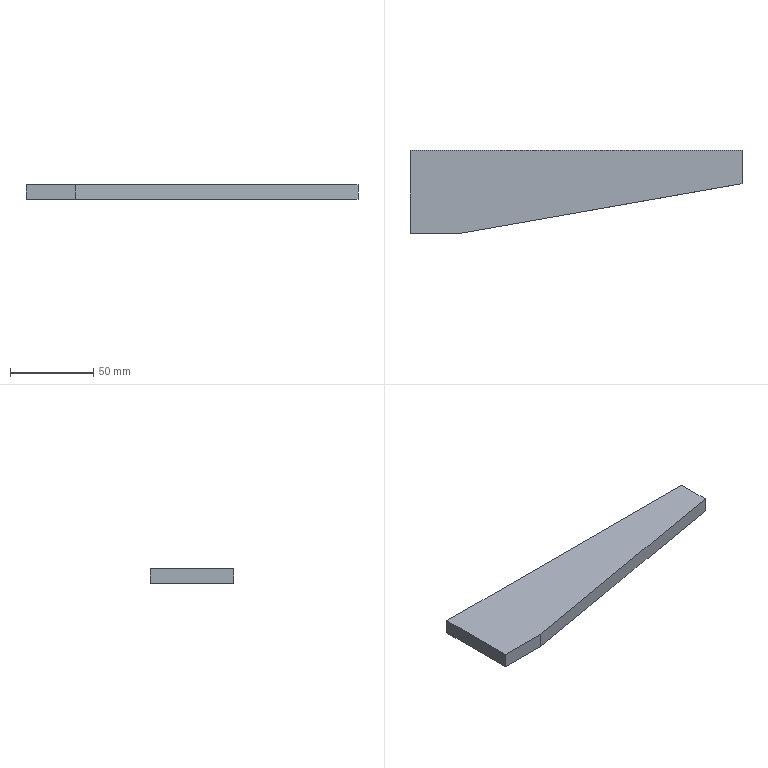Part | STEP file | [05]-1 | 1 solid | 7 faces | box 200 x 50 x 9 mm | volume 67050 mm3 | plane 7
STEP:
#1=CARTESIAN_POINT('',(0.,0.,0.));
#2=DIRECTION('',(0.,0.,1.));
#3=DIRECTION('',(1.,0.,0.));
#4=AXIS2_PLACEMENT_3D('',#1,#2,#3);
#5=CARTESIAN_POINT('',(200.,-20.,0.));
#6=VERTEX_POINT('',#5);
#7=CARTESIAN_POINT('',(200.,0.,0.));
#8=VERTEX_POINT('',#7);
#9=CARTESIAN_POINT('',(200.,-25.,0.));
#10=DIRECTION('',(0.,1.,0.));
#11=VECTOR('',#10,1.);
#12=LINE('',#9,#11);
#13=CARTESIAN_POINT('',(100.,-25.,0.));
#14=DIRECTION('',(0.,0.,-1.));
#15=DIRECTION('',(-1.,0.,0.));
#16=AXIS2_PLACEMENT_3D('',#13,#14,#15);
#17=PLANE('',#16);
#18=CARTESIAN_POINT('',(-100.,0.));
#19=DIRECTION('',(0.,1.));
#20=VECTOR('',#19,1.);
#21=LINE('',#18,#20);
#22=(GEOMETRIC_REPRESENTATION_CONTEXT(2)PARAMETRIC_REPRESENTATION_CONTEXT()REPRESENTATION_CONTEXT('',''));
#23=DEFINITIONAL_REPRESENTATION('',(#21),#22);
#24=PCURVE('',#17,#23);
#25=CARTESIAN_POINT('',(200.,-25.,9.));
#26=DIRECTION('',(1.,0.,0.));
#27=DIRECTION('',(0.,0.,-1.));
#28=AXIS2_PLACEMENT_3D('',#25,#26,#27);
#29=PLANE('',#28);
#30=CARTESIAN_POINT('',(9.,0.));
#31=DIRECTION('',(0.,1.));
#32=VECTOR('',#31,1.);
#33=LINE('',#30,#32);
#34=(GEOMETRIC_REPRESENTATION_CONTEXT(2)PARAMETRIC_REPRESENTATION_CONTEXT()REPRESENTATION_CONTEXT('',''));
#35=DEFINITIONAL_REPRESENTATION('',(#33),#34);
#36=PCURVE('',#29,#35);
#37=SURFACE_CURVE('',#12,(#24,#36),.PCURVE_S1.);
#38=EDGE_CURVE('',#6,#8,#37,.T.);
#39=ORIENTED_EDGE('',*,*,#38,.F.);
#40=CARTESIAN_POINT('',(30.,-50.,0.));
#41=VERTEX_POINT('',#40);
#42=CARTESIAN_POINT('',(102.164,-37.265,0.));
#43=DIRECTION('',(-0.9848,-0.1738,0.));
#44=VECTOR('',#43,1.);
#45=LINE('',#42,#44);
#46=CARTESIAN_POINT('',(-2.164,-12.265));
#47=DIRECTION('',(0.9848,-0.1738));
#48=VECTOR('',#47,1.);
#49=LINE('',#46,#48);
#50=(GEOMETRIC_REPRESENTATION_CONTEXT(2)PARAMETRIC_REPRESENTATION_CONTEXT()REPRESENTATION_CONTEXT('',''));
#51=DEFINITIONAL_REPRESENTATION('',(#49),#50);
#52=PCURVE('',#17,#51);
#53=CARTESIAN_POINT('',(200.,-20.,9.));
#54=DIRECTION('',(-0.1738,0.9848,0.));
#55=DIRECTION('',(0.,0.,-1.));
#56=AXIS2_PLACEMENT_3D('',#53,#54,#55);
#57=PLANE('',#56);
#58=CARTESIAN_POINT('',(9.,99.347));
#59=DIRECTION('',(0.,1.));
#60=VECTOR('',#59,1.);
#61=LINE('',#58,#60);
#62=(GEOMETRIC_REPRESENTATION_CONTEXT(2)PARAMETRIC_REPRESENTATION_CONTEXT()REPRESENTATION_CONTEXT('',''));
#63=DEFINITIONAL_REPRESENTATION('',(#61),#62);
#64=PCURVE('',#57,#63);
#65=SURFACE_CURVE('',#45,(#52,#64),.PCURVE_S1.);
#66=EDGE_CURVE('',#6,#41,#65,.T.);
#67=ORIENTED_EDGE('',*,*,#66,.T.);
#68=CARTESIAN_POINT('',(0.,-50.,0.));
#69=VERTEX_POINT('',#68);
#70=CARTESIAN_POINT('',(100.,-50.,0.));
#71=DIRECTION('',(1.,0.,0.));
#72=VECTOR('',#71,1.);
#73=LINE('',#70,#72);
#74=CARTESIAN_POINT('',(0.,-25.));
#75=DIRECTION('',(-1.,0.));
#76=VECTOR('',#75,1.);
#77=LINE('',#74,#76);
#78=(GEOMETRIC_REPRESENTATION_CONTEXT(2)PARAMETRIC_REPRESENTATION_CONTEXT()REPRESENTATION_CONTEXT('',''));
#79=DEFINITIONAL_REPRESENTATION('',(#77),#78);
#80=PCURVE('',#17,#79);
#81=CARTESIAN_POINT('',(100.,-50.,9.));
#82=DIRECTION('',(0.,-1.,0.));
#83=DIRECTION('',(0.,0.,1.));
#84=AXIS2_PLACEMENT_3D('',#81,#82,#83);
#85=PLANE('',#84);
#86=CARTESIAN_POINT('',(-9.,0.));
#87=DIRECTION('',(0.,-1.));
#88=VECTOR('',#87,1.);
#89=LINE('',#86,#88);
#90=(GEOMETRIC_REPRESENTATION_CONTEXT(2)PARAMETRIC_REPRESENTATION_CONTEXT()REPRESENTATION_CONTEXT('',''));
#91=DEFINITIONAL_REPRESENTATION('',(#89),#90);
#92=PCURVE('',#85,#91);
#93=SURFACE_CURVE('',#73,(#80,#92),.PCURVE_S1.);
#94=EDGE_CURVE('',#69,#41,#93,.T.);
#95=ORIENTED_EDGE('',*,*,#94,.F.);
#96=CARTESIAN_POINT('',(0.,0.,0.));
#97=VERTEX_POINT('',#96);
#98=CARTESIAN_POINT('',(0.,-25.,0.));
#99=DIRECTION('',(0.,-1.,0.));
#100=VECTOR('',#99,1.);
#101=LINE('',#98,#100);
#102=CARTESIAN_POINT('',(100.,0.));
#103=DIRECTION('',(0.,-1.));
#104=VECTOR('',#103,1.);
#105=LINE('',#102,#104);
#106=(GEOMETRIC_REPRESENTATION_CONTEXT(2)PARAMETRIC_REPRESENTATION_CONTEXT()REPRESENTATION_CONTEXT('',''));
#107=DEFINITIONAL_REPRESENTATION('',(#105),#106);
#108=PCURVE('',#17,#107);
#109=CARTESIAN_POINT('',(0.,-25.,9.));
#110=DIRECTION('',(-1.,0.,0.));
#111=DIRECTION('',(0.,0.,1.));
#112=AXIS2_PLACEMENT_3D('',#109,#110,#111);
#113=PLANE('',#112);
#114=CARTESIAN_POINT('',(-9.,0.));
#115=DIRECTION('',(0.,-1.));
#116=VECTOR('',#115,1.);
#117=LINE('',#114,#116);
#118=(GEOMETRIC_REPRESENTATION_CONTEXT(2)PARAMETRIC_REPRESENTATION_CONTEXT()REPRESENTATION_CONTEXT('',''));
#119=DEFINITIONAL_REPRESENTATION('',(#117),#118);
#120=PCURVE('',#113,#119);
#121=SURFACE_CURVE('',#101,(#108,#120),.PCURVE_S1.);
#122=EDGE_CURVE('',#97,#69,#121,.T.);
#123=ORIENTED_EDGE('',*,*,#122,.F.);
#124=CARTESIAN_POINT('',(100.,0.,0.));
#125=DIRECTION('',(-1.,0.,0.));
#126=VECTOR('',#125,1.);
#127=LINE('',#124,#126);
#128=CARTESIAN_POINT('',(0.,25.));
#129=DIRECTION('',(1.,0.));
#130=VECTOR('',#129,1.);
#131=LINE('',#128,#130);
#132=(GEOMETRIC_REPRESENTATION_CONTEXT(2)PARAMETRIC_REPRESENTATION_CONTEXT()REPRESENTATION_CONTEXT('',''));
#133=DEFINITIONAL_REPRESENTATION('',(#131),#132);
#134=PCURVE('',#17,#133);
#135=CARTESIAN_POINT('',(100.,0.,9.));
#136=DIRECTION('',(0.,1.,0.));
#137=DIRECTION('',(0.,0.,-1.));
#138=AXIS2_PLACEMENT_3D('',#135,#136,#137);
#139=PLANE('',#138);
#140=CARTESIAN_POINT('',(9.,0.));
#141=DIRECTION('',(0.,1.));
#142=VECTOR('',#141,1.);
#143=LINE('',#140,#142);
#144=(GEOMETRIC_REPRESENTATION_CONTEXT(2)PARAMETRIC_REPRESENTATION_CONTEXT()REPRESENTATION_CONTEXT('',''));
#145=DEFINITIONAL_REPRESENTATION('',(#143),#144);
#146=PCURVE('',#139,#145);
#147=SURFACE_CURVE('',#127,(#134,#146),.PCURVE_S1.);
#148=EDGE_CURVE('',#8,#97,#147,.T.);
#149=ORIENTED_EDGE('',*,*,#148,.F.);
#150=EDGE_LOOP('',(#39,#67,#95,#123,#149));
#151=FACE_BOUND('',#150,.T.);
#152=ADVANCED_FACE('',(#151),#17,.T.);
#153=ORIENTED_EDGE('',*,*,#94,.T.);
#154=CARTESIAN_POINT('',(30.,-50.,9.));
#155=VERTEX_POINT('',#154);
#156=CARTESIAN_POINT('',(30.,-50.,9.));
#157=DIRECTION('',(0.,0.,1.));
#158=VECTOR('',#157,1.);
#159=LINE('',#156,#158);
#160=CARTESIAN_POINT('',(0.,70.));
#161=DIRECTION('',(1.,0.));
#162=VECTOR('',#161,1.);
#163=LINE('',#160,#162);
#164=(GEOMETRIC_REPRESENTATION_CONTEXT(2)PARAMETRIC_REPRESENTATION_CONTEXT()REPRESENTATION_CONTEXT('',''));
#165=DEFINITIONAL_REPRESENTATION('',(#163),#164);
#166=PCURVE('',#85,#165);
#167=CARTESIAN_POINT('',(0.,172.627));
#168=DIRECTION('',(-1.,0.));
#169=VECTOR('',#168,1.);
#170=LINE('',#167,#169);
#171=(GEOMETRIC_REPRESENTATION_CONTEXT(2)PARAMETRIC_REPRESENTATION_CONTEXT()REPRESENTATION_CONTEXT('',''));
#172=DEFINITIONAL_REPRESENTATION('',(#170),#171);
#173=PCURVE('',#57,#172);
#174=SURFACE_CURVE('',#159,(#166,#173),.PCURVE_S1.);
#175=EDGE_CURVE('',#41,#155,#174,.T.);
#176=ORIENTED_EDGE('',*,*,#175,.T.);
#177=CARTESIAN_POINT('',(0.,-50.,9.));
#178=VERTEX_POINT('',#177);
#179=CARTESIAN_POINT('',(100.,-50.,9.));
#180=DIRECTION('',(-1.,0.,0.));
#181=VECTOR('',#180,1.);
#182=LINE('',#179,#181);
#183=CARTESIAN_POINT('',(0.,0.));
#184=DIRECTION('',(0.,1.));
#185=VECTOR('',#184,1.);
#186=LINE('',#183,#185);
#187=(GEOMETRIC_REPRESENTATION_CONTEXT(2)PARAMETRIC_REPRESENTATION_CONTEXT()REPRESENTATION_CONTEXT('',''));
#188=DEFINITIONAL_REPRESENTATION('',(#186),#187);
#189=PCURVE('',#85,#188);
#190=CARTESIAN_POINT('',(100.,-25.,9.));
#191=DIRECTION('',(0.,0.,1.));
#192=DIRECTION('',(1.,0.,0.));
#193=AXIS2_PLACEMENT_3D('',#190,#191,#192);
#194=PLANE('',#193);
#195=CARTESIAN_POINT('',(0.,-25.));
#196=DIRECTION('',(-1.,0.));
#197=VECTOR('',#196,1.);
#198=LINE('',#195,#197);
#199=(GEOMETRIC_REPRESENTATION_CONTEXT(2)PARAMETRIC_REPRESENTATION_CONTEXT()REPRESENTATION_CONTEXT('',''));
#200=DEFINITIONAL_REPRESENTATION('',(#198),#199);
#201=PCURVE('',#194,#200);
#202=SURFACE_CURVE('',#182,(#189,#201),.PCURVE_S1.);
#203=EDGE_CURVE('',#155,#178,#202,.T.);
#204=ORIENTED_EDGE('',*,*,#203,.T.);
#205=CARTESIAN_POINT('',(0.,-50.,9.));
#206=DIRECTION('',(0.,0.,-1.));
#207=VECTOR('',#206,1.);
#208=LINE('',#205,#207);
#209=CARTESIAN_POINT('',(0.,100.));
#210=DIRECTION('',(-1.,0.));
#211=VECTOR('',#210,1.);
#212=LINE('',#209,#211);
#213=(GEOMETRIC_REPRESENTATION_CONTEXT(2)PARAMETRIC_REPRESENTATION_CONTEXT()REPRESENTATION_CONTEXT('',''));
#214=DEFINITIONAL_REPRESENTATION('',(#212),#213);
#215=PCURVE('',#85,#214);
#216=CARTESIAN_POINT('',(0.,-25.));
#217=DIRECTION('',(-1.,0.));
#218=VECTOR('',#217,1.);
#219=LINE('',#216,#218);
#220=(GEOMETRIC_REPRESENTATION_CONTEXT(2)PARAMETRIC_REPRESENTATION_CONTEXT()REPRESENTATION_CONTEXT('',''));
#221=DEFINITIONAL_REPRESENTATION('',(#219),#220);
#222=PCURVE('',#113,#221);
#223=SURFACE_CURVE('',#208,(#215,#222),.PCURVE_S1.);
#224=EDGE_CURVE('',#178,#69,#223,.T.);
#225=ORIENTED_EDGE('',*,*,#224,.T.);
#226=EDGE_LOOP('',(#153,#176,#204,#225));
#227=FACE_BOUND('',#226,.T.);
#228=ADVANCED_FACE('',(#227),#85,.T.);
#229=CARTESIAN_POINT('',(200.,0.,9.));
#230=VERTEX_POINT('',#229);
#231=CARTESIAN_POINT('',(200.,-20.,9.));
#232=VERTEX_POINT('',#231);
#233=CARTESIAN_POINT('',(200.,-25.,9.));
#234=DIRECTION('',(0.,-1.,0.));
#235=VECTOR('',#234,1.);
#236=LINE('',#233,#235);
#237=CARTESIAN_POINT('',(0.,0.));
#238=DIRECTION('',(0.,-1.));
#239=VECTOR('',#238,1.);
#240=LINE('',#237,#239);
#241=(GEOMETRIC_REPRESENTATION_CONTEXT(2)PARAMETRIC_REPRESENTATION_CONTEXT()REPRESENTATION_CONTEXT('',''));
#242=DEFINITIONAL_REPRESENTATION('',(#240),#241);
#243=PCURVE('',#29,#242);
#244=CARTESIAN_POINT('',(100.,0.));
#245=DIRECTION('',(0.,-1.));
#246=VECTOR('',#245,1.);
#247=LINE('',#244,#246);
#248=(GEOMETRIC_REPRESENTATION_CONTEXT(2)PARAMETRIC_REPRESENTATION_CONTEXT()REPRESENTATION_CONTEXT('',''));
#249=DEFINITIONAL_REPRESENTATION('',(#247),#248);
#250=PCURVE('',#194,#249);
#251=SURFACE_CURVE('',#236,(#243,#250),.PCURVE_S1.);
#252=EDGE_CURVE('',#230,#232,#251,.T.);
#253=ORIENTED_EDGE('',*,*,#252,.T.);
#254=CARTESIAN_POINT('',(200.,-20.,9.));
#255=DIRECTION('',(0.,0.,-1.));
#256=VECTOR('',#255,1.);
#257=LINE('',#254,#256);
#258=CARTESIAN_POINT('',(0.,5.));
#259=DIRECTION('',(1.,0.));
#260=VECTOR('',#259,1.);
#261=LINE('',#258,#260);
#262=(GEOMETRIC_REPRESENTATION_CONTEXT(2)PARAMETRIC_REPRESENTATION_CONTEXT()REPRESENTATION_CONTEXT('',''));
#263=DEFINITIONAL_REPRESENTATION('',(#261),#262);
#264=PCURVE('',#29,#263);
#265=CARTESIAN_POINT('',(0.,0.));
#266=DIRECTION('',(1.,0.));
#267=VECTOR('',#266,1.);
#268=LINE('',#265,#267);
#269=(GEOMETRIC_REPRESENTATION_CONTEXT(2)PARAMETRIC_REPRESENTATION_CONTEXT()REPRESENTATION_CONTEXT('',''));
#270=DEFINITIONAL_REPRESENTATION('',(#268),#269);
#271=PCURVE('',#57,#270);
#272=SURFACE_CURVE('',#257,(#264,#271),.PCURVE_S1.);
#273=EDGE_CURVE('',#232,#6,#272,.T.);
#274=ORIENTED_EDGE('',*,*,#273,.T.);
#275=ORIENTED_EDGE('',*,*,#38,.T.);
#276=CARTESIAN_POINT('',(200.,0.,9.));
#277=DIRECTION('',(0.,0.,-1.));
#278=VECTOR('',#277,1.);
#279=LINE('',#276,#278);
#280=CARTESIAN_POINT('',(0.,25.));
#281=DIRECTION('',(1.,0.));
#282=VECTOR('',#281,1.);
#283=LINE('',#280,#282);
#284=(GEOMETRIC_REPRESENTATION_CONTEXT(2)PARAMETRIC_REPRESENTATION_CONTEXT()REPRESENTATION_CONTEXT('',''));
#285=DEFINITIONAL_REPRESENTATION('',(#283),#284);
#286=PCURVE('',#29,#285);
#287=CARTESIAN_POINT('',(0.,-100.));
#288=DIRECTION('',(1.,0.));
#289=VECTOR('',#288,1.);
#290=LINE('',#287,#289);
#291=(GEOMETRIC_REPRESENTATION_CONTEXT(2)PARAMETRIC_REPRESENTATION_CONTEXT()REPRESENTATION_CONTEXT('',''));
#292=DEFINITIONAL_REPRESENTATION('',(#290),#291);
#293=PCURVE('',#139,#292);
#294=SURFACE_CURVE('',#279,(#286,#293),.PCURVE_S1.);
#295=EDGE_CURVE('',#230,#8,#294,.T.);
#296=ORIENTED_EDGE('',*,*,#295,.F.);
#297=EDGE_LOOP('',(#253,#274,#275,#296));
#298=FACE_BOUND('',#297,.T.);
#299=ADVANCED_FACE('',(#298),#29,.T.);
#300=ORIENTED_EDGE('',*,*,#295,.T.);
#301=ORIENTED_EDGE('',*,*,#148,.T.);
#302=CARTESIAN_POINT('',(0.,0.,9.));
#303=VERTEX_POINT('',#302);
#304=CARTESIAN_POINT('',(0.,0.,9.));
#305=DIRECTION('',(0.,0.,-1.));
#306=VECTOR('',#305,1.);
#307=LINE('',#304,#306);
#308=CARTESIAN_POINT('',(0.,100.));
#309=DIRECTION('',(1.,0.));
#310=VECTOR('',#309,1.);
#311=LINE('',#308,#310);
#312=(GEOMETRIC_REPRESENTATION_CONTEXT(2)PARAMETRIC_REPRESENTATION_CONTEXT()REPRESENTATION_CONTEXT('',''));
#313=DEFINITIONAL_REPRESENTATION('',(#311),#312);
#314=PCURVE('',#139,#313);
#315=CARTESIAN_POINT('',(0.,25.));
#316=DIRECTION('',(-1.,0.));
#317=VECTOR('',#316,1.);
#318=LINE('',#315,#317);
#319=(GEOMETRIC_REPRESENTATION_CONTEXT(2)PARAMETRIC_REPRESENTATION_CONTEXT()REPRESENTATION_CONTEXT('',''));
#320=DEFINITIONAL_REPRESENTATION('',(#318),#319);
#321=PCURVE('',#113,#320);
#322=SURFACE_CURVE('',#307,(#314,#321),.PCURVE_S1.);
#323=EDGE_CURVE('',#303,#97,#322,.T.);
#324=ORIENTED_EDGE('',*,*,#323,.F.);
#325=CARTESIAN_POINT('',(100.,0.,9.));
#326=DIRECTION('',(1.,0.,0.));
#327=VECTOR('',#326,1.);
#328=LINE('',#325,#327);
#329=CARTESIAN_POINT('',(0.,0.));
#330=DIRECTION('',(0.,-1.));
#331=VECTOR('',#330,1.);
#332=LINE('',#329,#331);
#333=(GEOMETRIC_REPRESENTATION_CONTEXT(2)PARAMETRIC_REPRESENTATION_CONTEXT()REPRESENTATION_CONTEXT('',''));
#334=DEFINITIONAL_REPRESENTATION('',(#332),#333);
#335=PCURVE('',#139,#334);
#336=CARTESIAN_POINT('',(0.,25.));
#337=DIRECTION('',(1.,0.));
#338=VECTOR('',#337,1.);
#339=LINE('',#336,#338);
#340=(GEOMETRIC_REPRESENTATION_CONTEXT(2)PARAMETRIC_REPRESENTATION_CONTEXT()REPRESENTATION_CONTEXT('',''));
#341=DEFINITIONAL_REPRESENTATION('',(#339),#340);
#342=PCURVE('',#194,#341);
#343=SURFACE_CURVE('',#328,(#335,#342),.PCURVE_S1.);
#344=EDGE_CURVE('',#303,#230,#343,.T.);
#345=ORIENTED_EDGE('',*,*,#344,.T.);
#346=EDGE_LOOP('',(#300,#301,#324,#345));
#347=FACE_BOUND('',#346,.T.);
#348=ADVANCED_FACE('',(#347),#139,.T.);
#349=ORIENTED_EDGE('',*,*,#203,.F.);
#350=CARTESIAN_POINT('',(102.164,-37.265,9.));
#351=DIRECTION('',(0.9848,0.1738,0.));
#352=VECTOR('',#351,1.);
#353=LINE('',#350,#352);
#354=CARTESIAN_POINT('',(2.164,-12.265));
#355=DIRECTION('',(0.9848,0.1738));
#356=VECTOR('',#355,1.);
#357=LINE('',#354,#356);
#358=(GEOMETRIC_REPRESENTATION_CONTEXT(2)PARAMETRIC_REPRESENTATION_CONTEXT()REPRESENTATION_CONTEXT('',''));
#359=DEFINITIONAL_REPRESENTATION('',(#357),#358);
#360=PCURVE('',#194,#359);
#361=CARTESIAN_POINT('',(0.,99.347));
#362=DIRECTION('',(0.,-1.));
#363=VECTOR('',#362,1.);
#364=LINE('',#361,#363);
#365=(GEOMETRIC_REPRESENTATION_CONTEXT(2)PARAMETRIC_REPRESENTATION_CONTEXT()REPRESENTATION_CONTEXT('',''));
#366=DEFINITIONAL_REPRESENTATION('',(#364),#365);
#367=PCURVE('',#57,#366);
#368=SURFACE_CURVE('',#353,(#360,#367),.PCURVE_S1.);
#369=EDGE_CURVE('',#155,#232,#368,.T.);
#370=ORIENTED_EDGE('',*,*,#369,.T.);
#371=ORIENTED_EDGE('',*,*,#252,.F.);
#372=ORIENTED_EDGE('',*,*,#344,.F.);
#373=CARTESIAN_POINT('',(0.,-25.,9.));
#374=DIRECTION('',(0.,1.,0.));
#375=VECTOR('',#374,1.);
#376=LINE('',#373,#375);
#377=CARTESIAN_POINT('',(-100.,0.));
#378=DIRECTION('',(0.,1.));
#379=VECTOR('',#378,1.);
#380=LINE('',#377,#379);
#381=(GEOMETRIC_REPRESENTATION_CONTEXT(2)PARAMETRIC_REPRESENTATION_CONTEXT()REPRESENTATION_CONTEXT('',''));
#382=DEFINITIONAL_REPRESENTATION('',(#380),#381);
#383=PCURVE('',#194,#382);
#384=CARTESIAN_POINT('',(0.,0.));
#385=DIRECTION('',(0.,1.));
#386=VECTOR('',#385,1.);
#387=LINE('',#384,#386);
#388=(GEOMETRIC_REPRESENTATION_CONTEXT(2)PARAMETRIC_REPRESENTATION_CONTEXT()REPRESENTATION_CONTEXT('',''));
#389=DEFINITIONAL_REPRESENTATION('',(#387),#388);
#390=PCURVE('',#113,#389);
#391=SURFACE_CURVE('',#376,(#383,#390),.PCURVE_S1.);
#392=EDGE_CURVE('',#178,#303,#391,.T.);
#393=ORIENTED_EDGE('',*,*,#392,.F.);
#394=EDGE_LOOP('',(#349,#370,#371,#372,#393));
#395=FACE_BOUND('',#394,.T.);
#396=ADVANCED_FACE('',(#395),#194,.T.);
#397=ORIENTED_EDGE('',*,*,#392,.T.);
#398=ORIENTED_EDGE('',*,*,#323,.T.);
#399=ORIENTED_EDGE('',*,*,#122,.T.);
#400=ORIENTED_EDGE('',*,*,#224,.F.);
#401=EDGE_LOOP('',(#397,#398,#399,#400));
#402=FACE_BOUND('',#401,.T.);
#403=ADVANCED_FACE('',(#402),#113,.T.);
#404=ORIENTED_EDGE('',*,*,#369,.F.);
#405=ORIENTED_EDGE('',*,*,#175,.F.);
#406=ORIENTED_EDGE('',*,*,#66,.F.);
#407=ORIENTED_EDGE('',*,*,#273,.F.);
#408=EDGE_LOOP('',(#404,#405,#406,#407));
#409=FACE_BOUND('',#408,.T.);
#410=ADVANCED_FACE('',(#409),#57,.F.);
#411=CLOSED_SHELL('',(#152,#228,#299,#348,#396,#403,#410));
#412=MANIFOLD_SOLID_BREP('',#411);
#413=(LENGTH_UNIT()NAMED_UNIT(*)SI_UNIT(.MILLI.,.METRE.));
#414=UNCERTAINTY_MEASURE_WITH_UNIT(LENGTH_MEASURE(0.0000001),#413,'','');
#415=(NAMED_UNIT(*)PLANE_ANGLE_UNIT()SI_UNIT($,.RADIAN.));
#416=(NAMED_UNIT(*)SI_UNIT($,.STERADIAN.)SOLID_ANGLE_UNIT());
#417=(GEOMETRIC_REPRESENTATION_CONTEXT(3)GLOBAL_UNCERTAINTY_ASSIGNED_CONTEXT((#414))GLOBAL_UNIT_ASSIGNED_CONTEXT((#413,#415,#416))REPRESENTATION_CONTEXT('',''));
#418=ADVANCED_BREP_SHAPE_REPRESENTATION('',(#4,#412),#417);